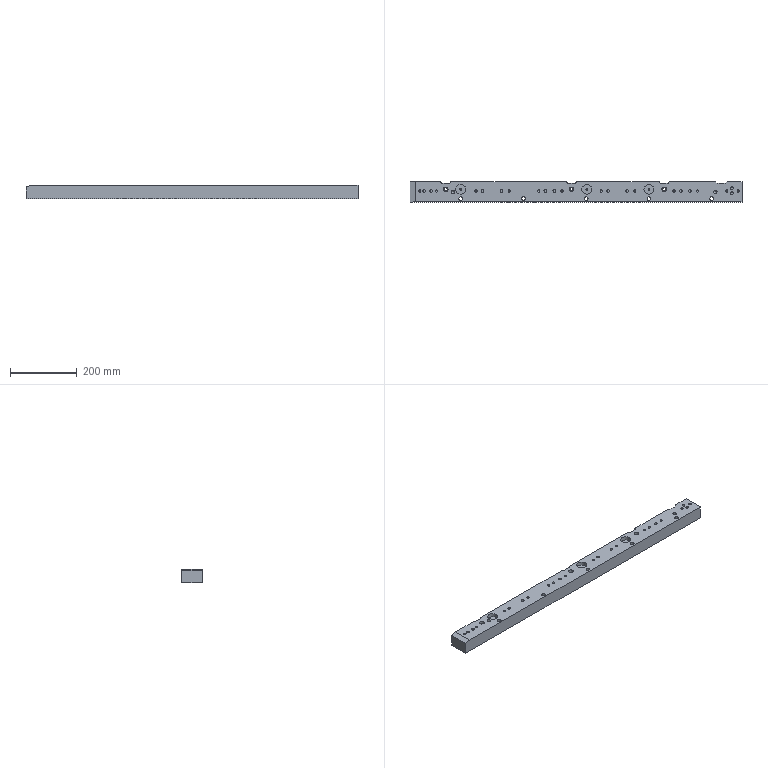Part | NX | features 22 2 | 1 solid | 114 faces | box 995 x 60 x 40 mm | volume 2257661 mm3 | cylinder 59 | plane 38 | cone 17 | commonest cylinder face diameters 6.8 x12 8.001 x12 14 x9 6 x6 11 x5 5.2 x3